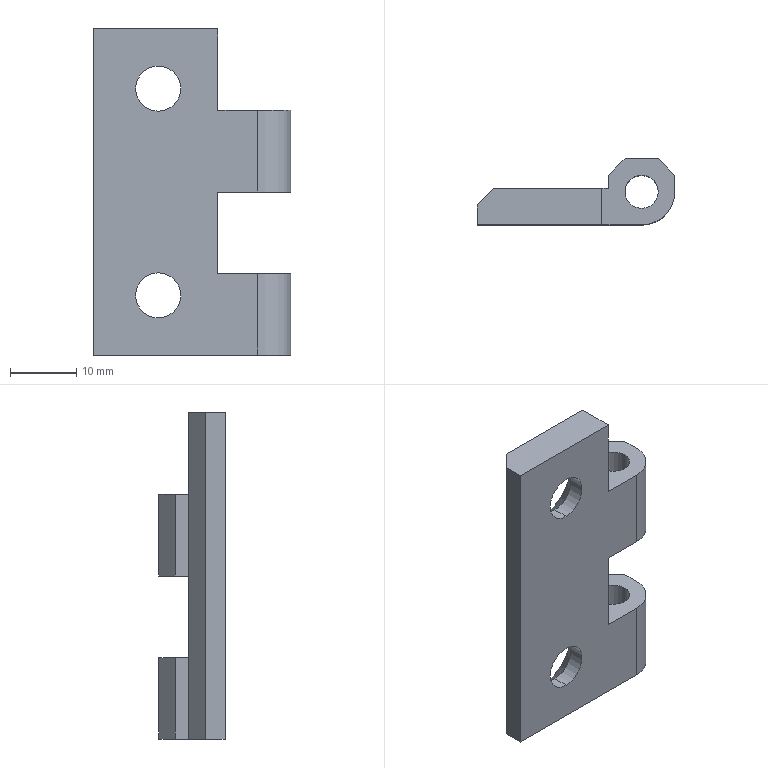Part | STEP file | Hinge CE-H3030-8-ZN | 1 solid | 35 faces | box 29.8 x 10 x 49.2 mm | volume 6093 mm3 | plane 21 | cylinder 10 | cone 4 | commonest cylinder face diameters 5 x4 6.8 x4 10 x2